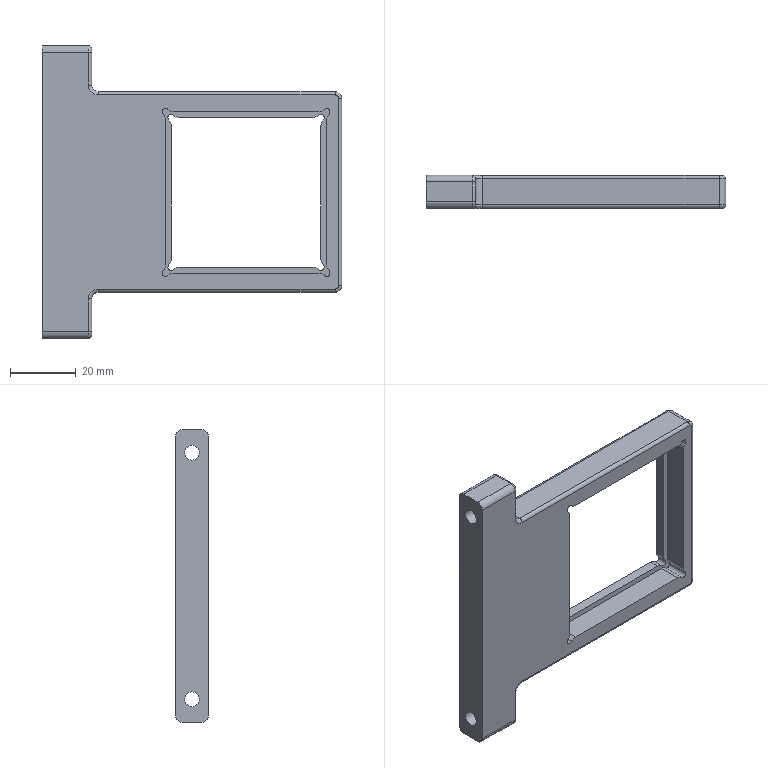Part | 1 solid | 83 faces | box 91 x 10 x 89 mm | volume 35532 mm3 | cylinder 48 | plane 23 | torus 12 | commonest cylinder face diameters 2 x20 5 x16 4 x8 4.5 x2 8 x2